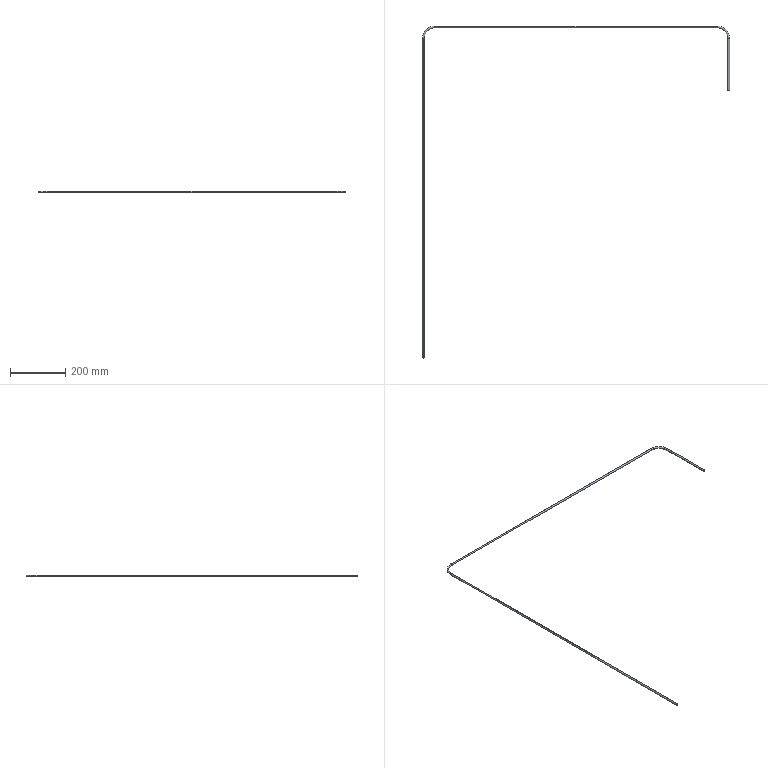Part | SolidWorks | features Sweep 1 | 1 solid | 12 faces | box 1109 x 1198 x 6.5 mm | volume 82657 mm3 | cylinder 6 | torus 4 | plane 2 | commonest cylinder face diameters 6.5 x6
STEP:
#1=CARTESIAN_POINT('',(1060.,1195.,-3.25));
#2=VERTEX_POINT('',#1);
#3=CARTESIAN_POINT('',(1060.,1198.25,0.));
#4=VERTEX_POINT('',#3);
#5=CARTESIAN_POINT('',(1060.,1195.,0.));
#6=DIRECTION('',(1.,0.,0.));
#7=DIRECTION('',(0.,0.,1.));
#8=AXIS2_PLACEMENT_3D('',#5,#6,#7);
#9=CIRCLE('',#8,3.25);
#10=EDGE_CURVE('',#2,#4,#9,.T.);
#11=ORIENTED_EDGE('',*,*,#10,.T.);
#12=CARTESIAN_POINT('',(1105.25,1153.,0.));
#13=VERTEX_POINT('',#12);
#14=CARTESIAN_POINT('',(1060.,1153.,0.));
#15=DIRECTION('',(0.,0.,-1.));
#16=DIRECTION('',(-1.,0.,0.));
#17=AXIS2_PLACEMENT_3D('',#14,#15,#16);
#18=CIRCLE('',#17,45.25);
#19=EDGE_CURVE('',#4,#13,#18,.T.);
#20=ORIENTED_EDGE('',*,*,#19,.T.);
#21=CARTESIAN_POINT('',(1098.75,1153.,0.));
#22=VERTEX_POINT('',#21);
#23=CARTESIAN_POINT('',(1102.,1153.,0.));
#24=DIRECTION('',(0.,-1.,0.));
#25=DIRECTION('',(0.,0.,1.));
#26=AXIS2_PLACEMENT_3D('',#23,#24,#25);
#27=CIRCLE('',#26,3.25);
#28=EDGE_CURVE('',#22,#13,#27,.T.);
#29=ORIENTED_EDGE('',*,*,#28,.F.);
#30=CARTESIAN_POINT('',(1060.,1191.75,0.));
#31=VERTEX_POINT('',#30);
#32=CARTESIAN_POINT('',(1060.,1153.,0.));
#33=DIRECTION('',(0.,0.,-1.));
#34=DIRECTION('',(-1.,0.,0.));
#35=AXIS2_PLACEMENT_3D('',#32,#33,#34);
#36=CIRCLE('',#35,38.75);
#37=EDGE_CURVE('',#31,#22,#36,.T.);
#38=ORIENTED_EDGE('',*,*,#37,.F.);
#39=CARTESIAN_POINT('',(1060.,1195.,0.));
#40=DIRECTION('',(1.,0.,0.));
#41=DIRECTION('',(0.,0.,1.));
#42=AXIS2_PLACEMENT_3D('',#39,#40,#41);
#43=CIRCLE('',#42,3.25);
#44=EDGE_CURVE('',#31,#2,#43,.T.);
#45=ORIENTED_EDGE('',*,*,#44,.T.);
#46=EDGE_LOOP('',(#11,#20,#29,#38,#45));
#47=FACE_OUTER_BOUND('',#46,.T.);
#48=CARTESIAN_POINT('',(1060.,1153.,0.));
#49=DIRECTION('',(0.,0.,-1.));
#50=DIRECTION('',(-1.,0.,0.));
#51=AXIS2_PLACEMENT_3D('',#48,#49,#50);
#52=TOROIDAL_SURFACE('',#51,42.,3.25);
#53=ADVANCED_FACE('',(#47),#52,.T.);
#54=CARTESIAN_POINT('',(0.,1153.,-3.25));
#55=VERTEX_POINT('',#54);
#56=CARTESIAN_POINT('',(-3.25,1153.,0.));
#57=VERTEX_POINT('',#56);
#58=CARTESIAN_POINT('',(0.,1153.,0.));
#59=DIRECTION('',(0.,1.,0.));
#60=DIRECTION('',(0.,0.,1.));
#61=AXIS2_PLACEMENT_3D('',#58,#59,#60);
#62=CIRCLE('',#61,3.25);
#63=EDGE_CURVE('',#55,#57,#62,.T.);
#64=ORIENTED_EDGE('',*,*,#63,.T.);
#65=CARTESIAN_POINT('',(42.,1198.25,0.));
#66=VERTEX_POINT('',#65);
#67=CARTESIAN_POINT('',(42.,1153.,0.));
#68=DIRECTION('',(0.,0.,-1.));
#69=DIRECTION('',(-1.,0.,0.));
#70=AXIS2_PLACEMENT_3D('',#67,#68,#69);
#71=CIRCLE('',#70,45.25);
#72=EDGE_CURVE('',#57,#66,#71,.T.);
#73=ORIENTED_EDGE('',*,*,#72,.T.);
#74=CARTESIAN_POINT('',(42.,1195.,-3.25));
#75=VERTEX_POINT('',#74);
#76=CARTESIAN_POINT('',(42.,1195.,0.));
#77=DIRECTION('',(1.,0.,0.));
#78=DIRECTION('',(0.,0.,1.));
#79=AXIS2_PLACEMENT_3D('',#76,#77,#78);
#80=CIRCLE('',#79,3.25);
#81=EDGE_CURVE('',#75,#66,#80,.T.);
#82=ORIENTED_EDGE('',*,*,#81,.F.);
#83=CARTESIAN_POINT('',(42.,1191.75,0.));
#84=VERTEX_POINT('',#83);
#85=CARTESIAN_POINT('',(42.,1195.,0.));
#86=DIRECTION('',(1.,0.,0.));
#87=DIRECTION('',(0.,0.,1.));
#88=AXIS2_PLACEMENT_3D('',#85,#86,#87);
#89=CIRCLE('',#88,3.25);
#90=EDGE_CURVE('',#84,#75,#89,.T.);
#91=ORIENTED_EDGE('',*,*,#90,.F.);
#92=CARTESIAN_POINT('',(3.25,1153.,0.));
#93=VERTEX_POINT('',#92);
#94=CARTESIAN_POINT('',(42.,1153.,0.));
#95=DIRECTION('',(0.,0.,-1.));
#96=DIRECTION('',(-1.,0.,0.));
#97=AXIS2_PLACEMENT_3D('',#94,#95,#96);
#98=CIRCLE('',#97,38.75);
#99=EDGE_CURVE('',#93,#84,#98,.T.);
#100=ORIENTED_EDGE('',*,*,#99,.F.);
#101=CARTESIAN_POINT('',(0.,1153.,0.));
#102=DIRECTION('',(0.,1.,0.));
#103=DIRECTION('',(0.,0.,1.));
#104=AXIS2_PLACEMENT_3D('',#101,#102,#103);
#105=CIRCLE('',#104,3.25);
#106=EDGE_CURVE('',#93,#55,#105,.T.);
#107=ORIENTED_EDGE('',*,*,#106,.T.);
#108=EDGE_LOOP('',(#64,#73,#82,#91,#100,#107));
#109=FACE_OUTER_BOUND('',#108,.T.);
#110=CARTESIAN_POINT('',(42.,1153.,0.));
#111=DIRECTION('',(0.,0.,-1.));
#112=DIRECTION('',(-1.,0.,0.));
#113=AXIS2_PLACEMENT_3D('',#110,#111,#112);
#114=TOROIDAL_SURFACE('',#113,42.,3.25);
#115=ADVANCED_FACE('',(#109),#114,.T.);
#116=CARTESIAN_POINT('',(1102.,1153.,0.));
#117=DIRECTION('',(0.,-1.,0.));
#118=DIRECTION('',(0.,0.,1.));
#119=AXIS2_PLACEMENT_3D('',#116,#117,#118);
#120=CIRCLE('',#119,3.25);
#121=EDGE_CURVE('',#13,#22,#120,.T.);
#122=ORIENTED_EDGE('',*,*,#121,.T.);
#123=CARTESIAN_POINT('',(1098.75,965.,0.));
#124=VERTEX_POINT('',#123);
#125=CARTESIAN_POINT('',(1098.75,1153.,0.));
#126=DIRECTION('',(0.,-1.,0.));
#127=VECTOR('',#126,1000.);
#128=LINE('',#125,#127);
#129=EDGE_CURVE('',#22,#124,#128,.T.);
#130=ORIENTED_EDGE('',*,*,#129,.T.);
#131=CARTESIAN_POINT('',(1105.25,965.,0.));
#132=VERTEX_POINT('',#131);
#133=CARTESIAN_POINT('',(1102.,965.,0.));
#134=DIRECTION('',(0.,-1.,0.));
#135=DIRECTION('',(0.,0.,1.));
#136=AXIS2_PLACEMENT_3D('',#133,#134,#135);
#137=CIRCLE('',#136,3.25);
#138=EDGE_CURVE('',#132,#124,#137,.T.);
#139=ORIENTED_EDGE('',*,*,#138,.F.);
#140=CARTESIAN_POINT('',(1105.25,1153.,0.));
#141=DIRECTION('',(0.,-1.,0.));
#142=VECTOR('',#141,1000.);
#143=LINE('',#140,#142);
#144=EDGE_CURVE('',#13,#132,#143,.T.);
#145=ORIENTED_EDGE('',*,*,#144,.F.);
#146=EDGE_LOOP('',(#122,#130,#139,#145));
#147=FACE_OUTER_BOUND('',#146,.T.);
#148=CARTESIAN_POINT('',(1102.,1153.,0.));
#149=DIRECTION('',(0.,-1.,0.));
#150=DIRECTION('',(1.,0.,0.));
#151=AXIS2_PLACEMENT_3D('',#148,#149,#150);
#152=CYLINDRICAL_SURFACE('',#151,3.25);
#153=ADVANCED_FACE('',(#147),#152,.T.);
#154=ORIENTED_EDGE('',*,*,#81,.T.);
#155=CARTESIAN_POINT('',(42.,1195.,3.25));
#156=VERTEX_POINT('',#155);
#157=CARTESIAN_POINT('',(42.,1195.,0.));
#158=DIRECTION('',(1.,0.,0.));
#159=DIRECTION('',(0.,0.,1.));
#160=AXIS2_PLACEMENT_3D('',#157,#158,#159);
#161=CIRCLE('',#160,3.25);
#162=EDGE_CURVE('',#66,#156,#161,.T.);
#163=ORIENTED_EDGE('',*,*,#162,.T.);
#164=CARTESIAN_POINT('',(1060.,1195.,3.25));
#165=VERTEX_POINT('',#164);
#166=CARTESIAN_POINT('',(42.,1195.,3.25));
#167=DIRECTION('',(1.,0.,0.));
#168=VECTOR('',#167,1000.);
#169=LINE('',#166,#168);
#170=EDGE_CURVE('',#156,#165,#169,.T.);
#171=ORIENTED_EDGE('',*,*,#170,.T.);
#172=CARTESIAN_POINT('',(1060.,1195.,0.));
#173=DIRECTION('',(1.,0.,0.));
#174=DIRECTION('',(0.,0.,1.));
#175=AXIS2_PLACEMENT_3D('',#172,#173,#174);
#176=CIRCLE('',#175,3.25);
#177=EDGE_CURVE('',#4,#165,#176,.T.);
#178=ORIENTED_EDGE('',*,*,#177,.F.);
#179=ORIENTED_EDGE('',*,*,#10,.F.);
#180=CARTESIAN_POINT('',(42.,1195.,-3.25));
#181=DIRECTION('',(1.,0.,0.));
#182=VECTOR('',#181,1000.);
#183=LINE('',#180,#182);
#184=EDGE_CURVE('',#75,#2,#183,.T.);
#185=ORIENTED_EDGE('',*,*,#184,.F.);
#186=EDGE_LOOP('',(#154,#163,#171,#178,#179,#185));
#187=FACE_OUTER_BOUND('',#186,.T.);
#188=CARTESIAN_POINT('',(42.,1195.,0.));
#189=DIRECTION('',(1.,0.,0.));
#190=DIRECTION('',(0.,0.,-1.));
#191=AXIS2_PLACEMENT_3D('',#188,#189,#190);
#192=CYLINDRICAL_SURFACE('',#191,3.25);
#193=ADVANCED_FACE('',(#187),#192,.T.);
#194=CARTESIAN_POINT('',(0.,0.,3.25));
#195=VERTEX_POINT('',#194);
#196=CARTESIAN_POINT('',(0.,0.,-3.25));
#197=VERTEX_POINT('',#196);
#198=CARTESIAN_POINT('',(0.,0.,0.));
#199=DIRECTION('',(0.,1.,0.));
#200=DIRECTION('',(0.,0.,1.));
#201=AXIS2_PLACEMENT_3D('',#198,#199,#200);
#202=CIRCLE('',#201,3.25);
#203=EDGE_CURVE('',#195,#197,#202,.T.);
#204=ORIENTED_EDGE('',*,*,#203,.T.);
#205=CARTESIAN_POINT('',(0.,0.,-3.25));
#206=DIRECTION('',(0.,1.,0.));
#207=VECTOR('',#206,1000.);
#208=LINE('',#205,#207);
#209=EDGE_CURVE('',#197,#55,#208,.T.);
#210=ORIENTED_EDGE('',*,*,#209,.T.);
#211=ORIENTED_EDGE('',*,*,#106,.F.);
#212=CARTESIAN_POINT('',(0.,1153.,3.25));
#213=VERTEX_POINT('',#212);
#214=CARTESIAN_POINT('',(0.,1153.,0.));
#215=DIRECTION('',(0.,1.,0.));
#216=DIRECTION('',(0.,0.,1.));
#217=AXIS2_PLACEMENT_3D('',#214,#215,#216);
#218=CIRCLE('',#217,3.25);
#219=EDGE_CURVE('',#213,#93,#218,.T.);
#220=ORIENTED_EDGE('',*,*,#219,.F.);
#221=CARTESIAN_POINT('',(0.,0.,3.25));
#222=DIRECTION('',(0.,1.,0.));
#223=VECTOR('',#222,1000.);
#224=LINE('',#221,#223);
#225=EDGE_CURVE('',#195,#213,#224,.T.);
#226=ORIENTED_EDGE('',*,*,#225,.F.);
#227=EDGE_LOOP('',(#204,#210,#211,#220,#226));
#228=FACE_OUTER_BOUND('',#227,.T.);
#229=CARTESIAN_POINT('',(0.,0.,0.));
#230=DIRECTION('',(0.,1.,0.));
#231=DIRECTION('',(0.,0.,1.));
#232=AXIS2_PLACEMENT_3D('',#229,#230,#231);
#233=CYLINDRICAL_SURFACE('',#232,3.25);
#234=ADVANCED_FACE('',(#228),#233,.T.);
#235=ORIENTED_EDGE('',*,*,#129,.F.);
#236=ORIENTED_EDGE('',*,*,#28,.T.);
#237=ORIENTED_EDGE('',*,*,#144,.T.);
#238=CARTESIAN_POINT('',(1102.,965.,0.));
#239=DIRECTION('',(0.,-1.,0.));
#240=DIRECTION('',(0.,0.,1.));
#241=AXIS2_PLACEMENT_3D('',#238,#239,#240);
#242=CIRCLE('',#241,3.25);
#243=EDGE_CURVE('',#124,#132,#242,.T.);
#244=ORIENTED_EDGE('',*,*,#243,.F.);
#245=EDGE_LOOP('',(#235,#236,#237,#244));
#246=FACE_OUTER_BOUND('',#245,.T.);
#247=CARTESIAN_POINT('',(1102.,1153.,0.));
#248=DIRECTION('',(0.,-1.,0.));
#249=DIRECTION('',(1.,0.,0.));
#250=AXIS2_PLACEMENT_3D('',#247,#248,#249);
#251=CYLINDRICAL_SURFACE('',#250,3.25);
#252=ADVANCED_FACE('',(#246),#251,.T.);
#253=ORIENTED_EDGE('',*,*,#19,.F.);
#254=ORIENTED_EDGE('',*,*,#177,.T.);
#255=CARTESIAN_POINT('',(1060.,1195.,0.));
#256=DIRECTION('',(1.,0.,0.));
#257=DIRECTION('',(0.,0.,1.));
#258=AXIS2_PLACEMENT_3D('',#255,#256,#257);
#259=CIRCLE('',#258,3.25);
#260=EDGE_CURVE('',#165,#31,#259,.T.);
#261=ORIENTED_EDGE('',*,*,#260,.T.);
#262=ORIENTED_EDGE('',*,*,#37,.T.);
#263=ORIENTED_EDGE('',*,*,#121,.F.);
#264=EDGE_LOOP('',(#253,#254,#261,#262,#263));
#265=FACE_OUTER_BOUND('',#264,.T.);
#266=CARTESIAN_POINT('',(1060.,1153.,0.));
#267=DIRECTION('',(0.,0.,-1.));
#268=DIRECTION('',(-1.,0.,0.));
#269=AXIS2_PLACEMENT_3D('',#266,#267,#268);
#270=TOROIDAL_SURFACE('',#269,42.,3.25);
#271=ADVANCED_FACE('',(#265),#270,.T.);
#272=ORIENTED_EDGE('',*,*,#170,.F.);
#273=CARTESIAN_POINT('',(42.,1195.,0.));
#274=DIRECTION('',(1.,0.,0.));
#275=DIRECTION('',(0.,0.,1.));
#276=AXIS2_PLACEMENT_3D('',#273,#274,#275);
#277=CIRCLE('',#276,3.25);
#278=EDGE_CURVE('',#156,#84,#277,.T.);
#279=ORIENTED_EDGE('',*,*,#278,.T.);
#280=ORIENTED_EDGE('',*,*,#90,.T.);
#281=ORIENTED_EDGE('',*,*,#184,.T.);
#282=ORIENTED_EDGE('',*,*,#44,.F.);
#283=ORIENTED_EDGE('',*,*,#260,.F.);
#284=EDGE_LOOP('',(#272,#279,#280,#281,#282,#283));
#285=FACE_OUTER_BOUND('',#284,.T.);
#286=CARTESIAN_POINT('',(42.,1195.,0.));
#287=DIRECTION('',(1.,0.,0.));
#288=DIRECTION('',(0.,0.,-1.));
#289=AXIS2_PLACEMENT_3D('',#286,#287,#288);
#290=CYLINDRICAL_SURFACE('',#289,3.25);
#291=ADVANCED_FACE('',(#285),#290,.T.);
#292=ORIENTED_EDGE('',*,*,#72,.F.);
#293=CARTESIAN_POINT('',(0.,1153.,0.));
#294=DIRECTION('',(0.,1.,0.));
#295=DIRECTION('',(0.,0.,1.));
#296=AXIS2_PLACEMENT_3D('',#293,#294,#295);
#297=CIRCLE('',#296,3.25);
#298=EDGE_CURVE('',#57,#213,#297,.T.);
#299=ORIENTED_EDGE('',*,*,#298,.T.);
#300=ORIENTED_EDGE('',*,*,#219,.T.);
#301=ORIENTED_EDGE('',*,*,#99,.T.);
#302=ORIENTED_EDGE('',*,*,#278,.F.);
#303=ORIENTED_EDGE('',*,*,#162,.F.);
#304=EDGE_LOOP('',(#292,#299,#300,#301,#302,#303));
#305=FACE_OUTER_BOUND('',#304,.T.);
#306=CARTESIAN_POINT('',(42.,1153.,0.));
#307=DIRECTION('',(0.,0.,-1.));
#308=DIRECTION('',(-1.,0.,0.));
#309=AXIS2_PLACEMENT_3D('',#306,#307,#308);
#310=TOROIDAL_SURFACE('',#309,42.,3.25);
#311=ADVANCED_FACE('',(#305),#310,.T.);
#312=ORIENTED_EDGE('',*,*,#209,.F.);
#313=CARTESIAN_POINT('',(0.,0.,0.));
#314=DIRECTION('',(0.,1.,0.));
#315=DIRECTION('',(0.,0.,1.));
#316=AXIS2_PLACEMENT_3D('',#313,#314,#315);
#317=CIRCLE('',#316,3.25);
#318=EDGE_CURVE('',#197,#195,#317,.T.);
#319=ORIENTED_EDGE('',*,*,#318,.T.);
#320=ORIENTED_EDGE('',*,*,#225,.T.);
#321=ORIENTED_EDGE('',*,*,#298,.F.);
#322=ORIENTED_EDGE('',*,*,#63,.F.);
#323=EDGE_LOOP('',(#312,#319,#320,#321,#322));
#324=FACE_OUTER_BOUND('',#323,.T.);
#325=CARTESIAN_POINT('',(0.,0.,0.));
#326=DIRECTION('',(0.,1.,0.));
#327=DIRECTION('',(0.,0.,1.));
#328=AXIS2_PLACEMENT_3D('',#325,#326,#327);
#329=CYLINDRICAL_SURFACE('',#328,3.25);
#330=ADVANCED_FACE('',(#324),#329,.T.);
#331=ORIENTED_EDGE('',*,*,#138,.T.);
#332=ORIENTED_EDGE('',*,*,#243,.T.);
#333=EDGE_LOOP('',(#331,#332));
#334=FACE_OUTER_BOUND('',#333,.T.);
#335=CARTESIAN_POINT('',(1102.,965.,0.));
#336=DIRECTION('',(0.,-1.,0.));
#337=DIRECTION('',(0.,0.,1.));
#338=AXIS2_PLACEMENT_3D('',#335,#336,#337);
#339=PLANE('',#338);
#340=ADVANCED_FACE('',(#334),#339,.T.);
#341=ORIENTED_EDGE('',*,*,#203,.F.);
#342=ORIENTED_EDGE('',*,*,#318,.F.);
#343=EDGE_LOOP('',(#341,#342));
#344=FACE_OUTER_BOUND('',#343,.T.);
#345=CARTESIAN_POINT('',(0.,0.,0.));
#346=DIRECTION('',(0.,1.,0.));
#347=DIRECTION('',(0.,0.,1.));
#348=AXIS2_PLACEMENT_3D('',#345,#346,#347);
#349=PLANE('',#348);
#350=ADVANCED_FACE('',(#344),#349,.F.);
#351=CLOSED_SHELL('',(#53,#115,#153,#193,#234,#252,#271,#291,#311,#330,#340,#350));
#352=MANIFOLD_SOLID_BREP('',#351);
#353=CARTESIAN_POINT('',(0.,0.,0.));
#354=DIRECTION('',(0.,0.,1.));
#355=DIRECTION('',(1.,0.,0.));
#356=AXIS2_PLACEMENT_3D('',#353,#354,#355);
#357=(LENGTH_UNIT()NAMED_UNIT(*)SI_UNIT(.MILLI.,.METRE.));
#358=UNCERTAINTY_MEASURE_WITH_UNIT(LENGTH_MEASURE(0.00001),#357,'','');
#359=(NAMED_UNIT(*)PLANE_ANGLE_UNIT()SI_UNIT($,.RADIAN.));
#360=(NAMED_UNIT(*)SI_UNIT($,.STERADIAN.)SOLID_ANGLE_UNIT());
#361=(GEOMETRIC_REPRESENTATION_CONTEXT(3)GLOBAL_UNCERTAINTY_ASSIGNED_CONTEXT((#358))GLOBAL_UNIT_ASSIGNED_CONTEXT((#357,#359,#360))REPRESENTATION_CONTEXT('',''));
#362=ADVANCED_BREP_SHAPE_REPRESENTATION('',(#352,#356),#361);